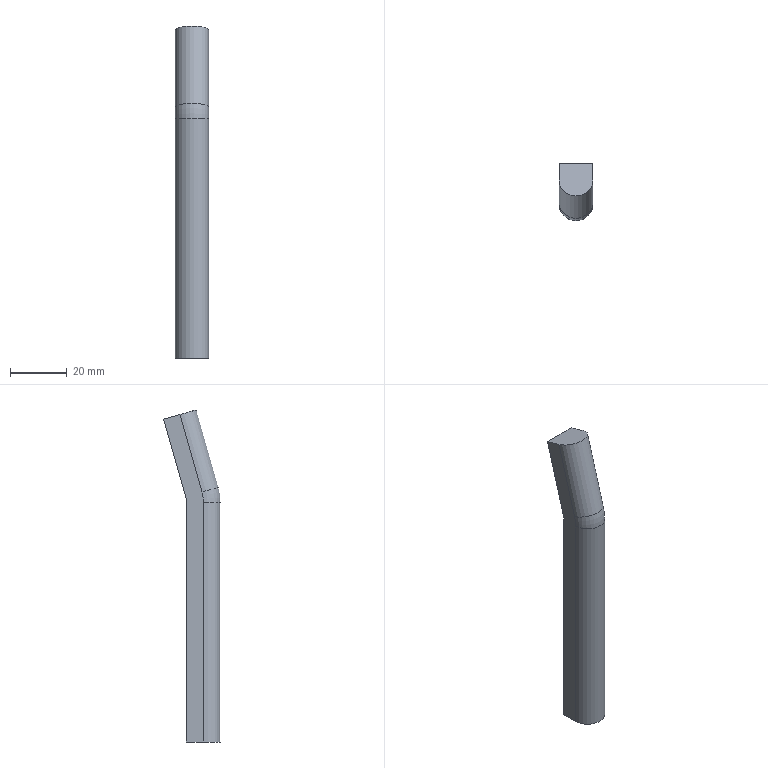Part | NX | features solid 2 | 1 solid | 10 faces | box 12 x 20.071 x 117.272 mm | volume 14990 mm3 | plane 6 | cylinder 3 | torus 1 | commonest cylinder face diameters 12 x2 16 x1
STEP:
#1=CARTESIAN_POINT('',(546.,577.,44.523));
#2=VERTEX_POINT('',#1);
#3=CARTESIAN_POINT('',(558.,577.,44.523));
#4=VERTEX_POINT('',#3);
#5=CARTESIAN_POINT('',(582.,577.,44.523));
#6=DIRECTION('',(1.,0.,0.));
#7=VECTOR('',#6,1000.);
#8=LINE('',#5,#7);
#9=EDGE_CURVE('',#2,#4,#8,.T.);
#10=ORIENTED_EDGE('',*,*,#9,.T.);
#11=CARTESIAN_POINT('',(558.,577.,-40.));
#12=VERTEX_POINT('',#11);
#13=CARTESIAN_POINT('',(558.,577.,79.523));
#14=DIRECTION('',(0.,0.,-1.));
#15=VECTOR('',#14,1000.);
#16=LINE('',#13,#15);
#17=EDGE_CURVE('',#4,#12,#16,.T.);
#18=ORIENTED_EDGE('',*,*,#17,.T.);
#19=CARTESIAN_POINT('',(546.,577.,-40.));
#20=VERTEX_POINT('',#19);
#21=CARTESIAN_POINT('',(525.,577.,-40.));
#22=DIRECTION('',(1.,0.,0.));
#23=VECTOR('',#22,1000.);
#24=LINE('',#21,#23);
#25=EDGE_CURVE('',#20,#12,#24,.T.);
#26=ORIENTED_EDGE('',*,*,#25,.F.);
#27=CARTESIAN_POINT('',(546.,577.,69.523));
#28=DIRECTION('',(0.,0.,-1.));
#29=VECTOR('',#28,1000.);
#30=LINE('',#27,#29);
#31=EDGE_CURVE('',#2,#20,#30,.T.);
#32=ORIENTED_EDGE('',*,*,#31,.F.);
#33=EDGE_LOOP('',(#10,#18,#26,#32));
#34=FACE_BOUND('',#33,.T.);
#35=CARTESIAN_POINT('',(582.,577.,79.523));
#36=DIRECTION('',(0.,-1.,0.));
#37=DIRECTION('',(-1.,0.,0.));
#38=AXIS2_PLACEMENT_3D('',#35,#36,#37);
#39=PLANE('',#38);
#40=ADVANCED_FACE('',(#34),#39,.F.);
#41=CARTESIAN_POINT('',(558.,571.,44.523));
#42=VERTEX_POINT('',#41);
#43=CARTESIAN_POINT('',(546.,571.,44.523));
#44=VERTEX_POINT('',#43);
#45=CARTESIAN_POINT('',(552.,571.,44.523));
#46=DIRECTION('',(0.,0.,-1.));
#47=DIRECTION('',(0.,-1.,0.));
#48=AXIS2_PLACEMENT_3D('',#45,#46,#47);
#49=CIRCLE('',#48,6.);
#50=EDGE_CURVE('',#42,#44,#49,.T.);
#51=ORIENTED_EDGE('',*,*,#50,.F.);
#52=CARTESIAN_POINT('',(558.,571.535,48.357));
#53=VERTEX_POINT('',#52);
#54=CARTESIAN_POINT('',(558.,585.,44.523));
#55=DIRECTION('',(-1.,0.,0.));
#56=DIRECTION('',(0.,0.,-1.));
#57=AXIS2_PLACEMENT_3D('',#54,#55,#56);
#58=CIRCLE('',#57,14.);
#59=EDGE_CURVE('',#42,#53,#58,.T.);
#60=ORIENTED_EDGE('',*,*,#59,.T.);
#61=CARTESIAN_POINT('',(546.,571.535,48.357));
#62=VERTEX_POINT('',#61);
#63=CARTESIAN_POINT('',(552.,571.535,48.357));
#64=DIRECTION('',(0.,-0.2738,-0.9618));
#65=DIRECTION('',(0.,-0.9618,0.2738));
#66=AXIS2_PLACEMENT_3D('',#63,#64,#65);
#67=CIRCLE('',#66,6.);
#68=EDGE_CURVE('',#53,#62,#67,.T.);
#69=ORIENTED_EDGE('',*,*,#68,.T.);
#70=CARTESIAN_POINT('',(546.,585.,44.523));
#71=DIRECTION('',(-1.,0.,0.));
#72=DIRECTION('',(0.,0.,-1.));
#73=AXIS2_PLACEMENT_3D('',#70,#71,#72);
#74=CIRCLE('',#73,14.);
#75=EDGE_CURVE('',#44,#62,#74,.T.);
#76=ORIENTED_EDGE('',*,*,#75,.F.);
#77=EDGE_LOOP('',(#51,#60,#69,#76));
#78=FACE_BOUND('',#77,.T.);
#79=CARTESIAN_POINT('',(552.,585.,44.523));
#80=DIRECTION('',(1.,0.,0.));
#81=DIRECTION('',(0.,0.,-1.));
#82=AXIS2_PLACEMENT_3D('',#79,#80,#81);
#83=TOROIDAL_SURFACE('',#82,14.,6.);
#84=ADVANCED_FACE('',(#78),#83,.T.);
#85=CARTESIAN_POINT('',(558.,579.3,75.629));
#86=VERTEX_POINT('',#85);
#87=CARTESIAN_POINT('',(558.,571.535,48.357));
#88=DIRECTION('',(0.,0.2738,0.9618));
#89=VECTOR('',#88,1000.);
#90=LINE('',#87,#89);
#91=EDGE_CURVE('',#53,#86,#90,.T.);
#92=ORIENTED_EDGE('',*,*,#91,.T.);
#93=CARTESIAN_POINT('',(546.,579.3,75.629));
#94=VERTEX_POINT('',#93);
#95=CARTESIAN_POINT('',(552.,579.3,75.629));
#96=DIRECTION('',(0.,0.2738,0.9618));
#97=DIRECTION('',(0.,-0.9618,0.2738));
#98=AXIS2_PLACEMENT_3D('',#95,#96,#97);
#99=CIRCLE('',#98,6.);
#100=EDGE_CURVE('',#86,#94,#99,.F.);
#101=ORIENTED_EDGE('',*,*,#100,.T.);
#102=CARTESIAN_POINT('',(546.,571.535,48.357));
#103=DIRECTION('',(0.,0.2738,0.9618));
#104=VECTOR('',#103,1000.);
#105=LINE('',#102,#104);
#106=EDGE_CURVE('',#62,#94,#105,.T.);
#107=ORIENTED_EDGE('',*,*,#106,.F.);
#108=ORIENTED_EDGE('',*,*,#68,.F.);
#109=EDGE_LOOP('',(#92,#101,#107,#108));
#110=FACE_BOUND('',#109,.T.);
#111=CARTESIAN_POINT('',(552.,571.535,48.357));
#112=DIRECTION('',(0.,0.2738,0.9618));
#113=DIRECTION('',(0.,-0.9618,0.2738));
#114=AXIS2_PLACEMENT_3D('',#111,#112,#113);
#115=CYLINDRICAL_SURFACE('',#114,6.);
#116=ADVANCED_FACE('',(#110),#115,.T.);
#117=ORIENTED_EDGE('',*,*,#100,.F.);
#118=CARTESIAN_POINT('',(558.,585.071,73.986));
#119=VERTEX_POINT('',#118);
#120=CARTESIAN_POINT('',(558.,586.81,73.491));
#121=DIRECTION('',(0.,0.9618,-0.2738));
#122=VECTOR('',#121,1000.);
#123=LINE('',#120,#122);
#124=EDGE_CURVE('',#86,#119,#123,.T.);
#125=ORIENTED_EDGE('',*,*,#124,.T.);
#126=CARTESIAN_POINT('',(546.,585.071,73.986));
#127=VERTEX_POINT('',#126);
#128=CARTESIAN_POINT('',(582.,585.071,73.986));
#129=DIRECTION('',(1.,0.,0.));
#130=VECTOR('',#129,1000.);
#131=LINE('',#128,#130);
#132=EDGE_CURVE('',#127,#119,#131,.T.);
#133=ORIENTED_EDGE('',*,*,#132,.F.);
#134=CARTESIAN_POINT('',(546.,586.81,73.491));
#135=DIRECTION('',(0.,0.9618,-0.2738));
#136=VECTOR('',#135,1000.);
#137=LINE('',#134,#136);
#138=EDGE_CURVE('',#94,#127,#137,.T.);
#139=ORIENTED_EDGE('',*,*,#138,.F.);
#140=EDGE_LOOP('',(#117,#125,#133,#139));
#141=FACE_BOUND('',#140,.T.);
#142=CARTESIAN_POINT('',(611.75,586.81,73.491));
#143=DIRECTION('',(0.,0.2738,0.9618));
#144=DIRECTION('',(0.,-0.9618,0.2738));
#145=AXIS2_PLACEMENT_3D('',#142,#143,#144);
#146=PLANE('',#145);
#147=ADVANCED_FACE('',(#141),#146,.T.);
#148=ORIENTED_EDGE('',*,*,#17,.F.);
#149=CARTESIAN_POINT('',(558.,577.306,46.714));
#150=VERTEX_POINT('',#149);
#151=CARTESIAN_POINT('',(558.,585.,44.523));
#152=DIRECTION('',(-1.,0.,0.));
#153=DIRECTION('',(0.,0.,-1.));
#154=AXIS2_PLACEMENT_3D('',#151,#152,#153);
#155=CIRCLE('',#154,8.);
#156=EDGE_CURVE('',#4,#150,#155,.T.);
#157=ORIENTED_EDGE('',*,*,#156,.T.);
#158=CARTESIAN_POINT('',(558.,577.306,46.714));
#159=DIRECTION('',(0.,0.2738,0.9618));
#160=VECTOR('',#159,1000.);
#161=LINE('',#158,#160);
#162=EDGE_CURVE('',#150,#119,#161,.T.);
#163=ORIENTED_EDGE('',*,*,#162,.T.);
#164=ORIENTED_EDGE('',*,*,#124,.F.);
#165=ORIENTED_EDGE('',*,*,#91,.F.);
#166=ORIENTED_EDGE('',*,*,#59,.F.);
#167=CARTESIAN_POINT('',(558.,571.,-40.));
#168=VERTEX_POINT('',#167);
#169=CARTESIAN_POINT('',(558.,571.,59.523));
#170=DIRECTION('',(0.,0.,-1.));
#171=VECTOR('',#170,1000.);
#172=LINE('',#169,#171);
#173=EDGE_CURVE('',#42,#168,#172,.T.);
#174=ORIENTED_EDGE('',*,*,#173,.T.);
#175=CARTESIAN_POINT('',(558.,669.,-40.));
#176=DIRECTION('',(0.,1.,0.));
#177=VECTOR('',#176,1000.);
#178=LINE('',#175,#177);
#179=EDGE_CURVE('',#168,#12,#178,.T.);
#180=ORIENTED_EDGE('',*,*,#179,.T.);
#181=EDGE_LOOP('',(#148,#157,#163,#164,#165,#166,#174,#180));
#182=FACE_BOUND('',#181,.T.);
#183=CARTESIAN_POINT('',(558.,669.,69.523));
#184=DIRECTION('',(1.,0.,0.));
#185=DIRECTION('',(0.,-1.,0.));
#186=AXIS2_PLACEMENT_3D('',#183,#184,#185);
#187=PLANE('',#186);
#188=ADVANCED_FACE('',(#182),#187,.T.);
#189=ORIENTED_EDGE('',*,*,#106,.T.);
#190=ORIENTED_EDGE('',*,*,#138,.T.);
#191=CARTESIAN_POINT('',(546.,577.306,46.714));
#192=VERTEX_POINT('',#191);
#193=CARTESIAN_POINT('',(546.,577.306,46.714));
#194=DIRECTION('',(0.,0.2738,0.9618));
#195=VECTOR('',#194,1000.);
#196=LINE('',#193,#195);
#197=EDGE_CURVE('',#192,#127,#196,.T.);
#198=ORIENTED_EDGE('',*,*,#197,.F.);
#199=CARTESIAN_POINT('',(546.,585.,44.523));
#200=DIRECTION('',(-1.,0.,0.));
#201=DIRECTION('',(0.,0.,-1.));
#202=AXIS2_PLACEMENT_3D('',#199,#200,#201);
#203=CIRCLE('',#202,8.);
#204=EDGE_CURVE('',#2,#192,#203,.T.);
#205=ORIENTED_EDGE('',*,*,#204,.F.);
#206=ORIENTED_EDGE('',*,*,#31,.T.);
#207=CARTESIAN_POINT('',(546.,571.,-40.));
#208=VERTEX_POINT('',#207);
#209=CARTESIAN_POINT('',(546.,669.,-40.));
#210=DIRECTION('',(0.,1.,0.));
#211=VECTOR('',#210,1000.);
#212=LINE('',#209,#211);
#213=EDGE_CURVE('',#208,#20,#212,.T.);
#214=ORIENTED_EDGE('',*,*,#213,.F.);
#215=CARTESIAN_POINT('',(546.,571.,59.523));
#216=DIRECTION('',(0.,0.,-1.));
#217=VECTOR('',#216,1000.);
#218=LINE('',#215,#217);
#219=EDGE_CURVE('',#44,#208,#218,.T.);
#220=ORIENTED_EDGE('',*,*,#219,.F.);
#221=ORIENTED_EDGE('',*,*,#75,.T.);
#222=EDGE_LOOP('',(#189,#190,#198,#205,#206,#214,#220,#221));
#223=FACE_BOUND('',#222,.T.);
#224=CARTESIAN_POINT('',(546.,669.,69.523));
#225=DIRECTION('',(1.,0.,0.));
#226=DIRECTION('',(0.,-1.,0.));
#227=AXIS2_PLACEMENT_3D('',#224,#225,#226);
#228=PLANE('',#227);
#229=ADVANCED_FACE('',(#223),#228,.F.);
#230=ORIENTED_EDGE('',*,*,#219,.T.);
#231=CARTESIAN_POINT('',(552.,571.,-40.));
#232=DIRECTION('',(0.,0.,-1.));
#233=DIRECTION('',(-1.,0.,0.));
#234=AXIS2_PLACEMENT_3D('',#231,#232,#233);
#235=CIRCLE('',#234,6.);
#236=EDGE_CURVE('',#168,#208,#235,.T.);
#237=ORIENTED_EDGE('',*,*,#236,.F.);
#238=ORIENTED_EDGE('',*,*,#173,.F.);
#239=ORIENTED_EDGE('',*,*,#50,.T.);
#240=EDGE_LOOP('',(#230,#237,#238,#239));
#241=FACE_BOUND('',#240,.T.);
#242=CARTESIAN_POINT('',(552.,571.,59.523));
#243=DIRECTION('',(0.,0.,-1.));
#244=DIRECTION('',(0.,1.,0.));
#245=AXIS2_PLACEMENT_3D('',#242,#243,#244);
#246=CYLINDRICAL_SURFACE('',#245,6.);
#247=ADVANCED_FACE('',(#241),#246,.T.);
#248=ORIENTED_EDGE('',*,*,#213,.T.);
#249=ORIENTED_EDGE('',*,*,#25,.T.);
#250=ORIENTED_EDGE('',*,*,#179,.F.);
#251=ORIENTED_EDGE('',*,*,#236,.T.);
#252=EDGE_LOOP('',(#248,#249,#250,#251));
#253=FACE_BOUND('',#252,.T.);
#254=CARTESIAN_POINT('',(525.,602.,-40.));
#255=DIRECTION('',(0.,0.,1.));
#256=DIRECTION('',(1.,0.,0.));
#257=AXIS2_PLACEMENT_3D('',#254,#255,#256);
#258=PLANE('',#257);
#259=ADVANCED_FACE('',(#253),#258,.F.);
#260=CARTESIAN_POINT('',(582.,577.306,46.714));
#261=DIRECTION('',(1.,0.,0.));
#262=VECTOR('',#261,1000.);
#263=LINE('',#260,#262);
#264=EDGE_CURVE('',#192,#150,#263,.T.);
#265=ORIENTED_EDGE('',*,*,#264,.F.);
#266=ORIENTED_EDGE('',*,*,#197,.T.);
#267=ORIENTED_EDGE('',*,*,#132,.T.);
#268=ORIENTED_EDGE('',*,*,#162,.F.);
#269=EDGE_LOOP('',(#265,#266,#267,#268));
#270=FACE_BOUND('',#269,.T.);
#271=CARTESIAN_POINT('',(582.,577.306,46.714));
#272=DIRECTION('',(0.,0.9618,-0.2738));
#273=DIRECTION('',(0.,0.2738,0.9618));
#274=AXIS2_PLACEMENT_3D('',#271,#272,#273);
#275=PLANE('',#274);
#276=ADVANCED_FACE('',(#270),#275,.T.);
#277=ORIENTED_EDGE('',*,*,#9,.F.);
#278=ORIENTED_EDGE('',*,*,#204,.T.);
#279=ORIENTED_EDGE('',*,*,#264,.T.);
#280=ORIENTED_EDGE('',*,*,#156,.F.);
#281=EDGE_LOOP('',(#277,#278,#279,#280));
#282=FACE_BOUND('',#281,.T.);
#283=CARTESIAN_POINT('',(597.,585.,44.523));
#284=DIRECTION('',(1.,0.,0.));
#285=DIRECTION('',(0.,0.,-1.));
#286=AXIS2_PLACEMENT_3D('',#283,#284,#285);
#287=CYLINDRICAL_SURFACE('',#286,8.);
#288=ADVANCED_FACE('',(#282),#287,.F.);
#289=CLOSED_SHELL('',(#40,#84,#116,#147,#188,#229,#247,#259,#276,#288));
#290=MANIFOLD_SOLID_BREP('',#289);
#291=(LENGTH_UNIT()NAMED_UNIT(*)SI_UNIT(.MILLI.,.METRE.));
#292=UNCERTAINTY_MEASURE_WITH_UNIT(LENGTH_MEASURE(0.00001),#291,'','');
#293=(NAMED_UNIT(*)PLANE_ANGLE_UNIT()SI_UNIT($,.RADIAN.));
#294=(NAMED_UNIT(*)SI_UNIT($,.STERADIAN.)SOLID_ANGLE_UNIT());
#295=(GEOMETRIC_REPRESENTATION_CONTEXT(3)GLOBAL_UNCERTAINTY_ASSIGNED_CONTEXT((#292))GLOBAL_UNIT_ASSIGNED_CONTEXT((#291,#293,#294))REPRESENTATION_CONTEXT('',''));
#296=ADVANCED_BREP_SHAPE_REPRESENTATION('',(#290),#295);